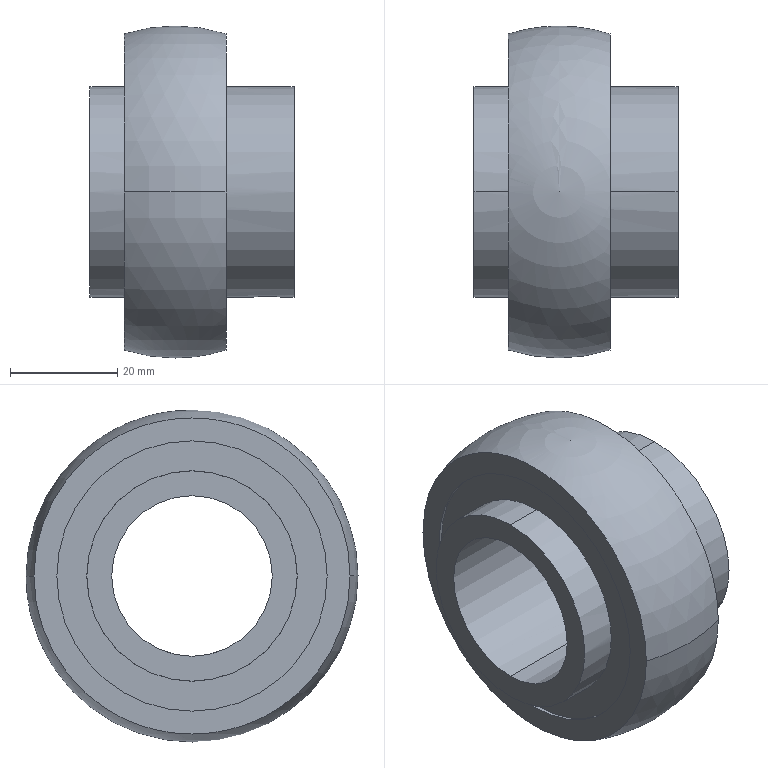Part | SolidWorks | features Revolution 3, RevCut 2, CirPattern 1 | 1 solid | 37 faces | box 38.1 x 62 x 62 mm | volume 38211 mm3 | cylinder 18 | sphere 10 | plane 9 | commonest cylinder face diameters 50.48 x6 39.3 x4 2.5 x2 5.351 x2 30 x2 39.28 x2